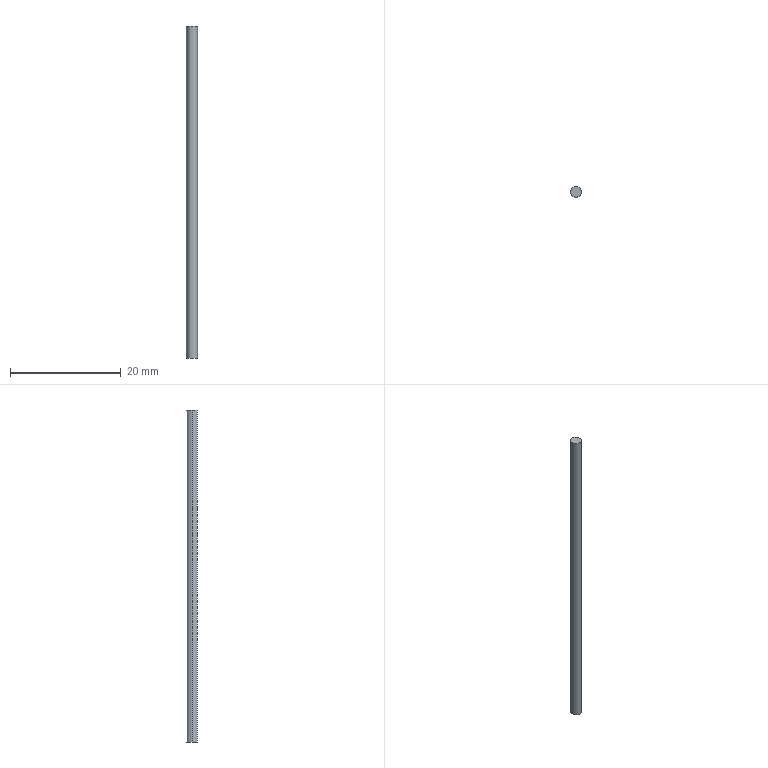Part | SolidWorks | features Extrusion 1 | 1 solid | 4 faces | box 2 x 2 x 60 mm | volume 188.496 mm3 | cylinder 2 | plane 2 | commonest cylinder face diameters 2 x2
STEP:
#1=CARTESIAN_POINT('',(1.,0.,60.));
#2=VERTEX_POINT('',#1);
#3=CARTESIAN_POINT('',(-1.,0.,60.));
#4=VERTEX_POINT('',#3);
#5=CARTESIAN_POINT('',(0.,0.,60.));
#6=DIRECTION('',(0.,0.,1.));
#7=DIRECTION('',(1.,0.,0.));
#8=AXIS2_PLACEMENT_3D('',#5,#6,#7);
#9=CIRCLE('',#8,1.);
#10=EDGE_CURVE('',#2,#4,#9,.T.);
#11=ORIENTED_EDGE('',*,*,#10,.F.);
#12=CARTESIAN_POINT('',(1.,0.,0.));
#13=VERTEX_POINT('',#12);
#14=CARTESIAN_POINT('',(1.,0.,60.));
#15=DIRECTION('',(0.,0.,-1.));
#16=VECTOR('',#15,1000.);
#17=LINE('',#14,#16);
#18=EDGE_CURVE('',#2,#13,#17,.T.);
#19=ORIENTED_EDGE('',*,*,#18,.T.);
#20=CARTESIAN_POINT('',(-1.,0.,0.));
#21=VERTEX_POINT('',#20);
#22=CARTESIAN_POINT('',(0.,0.,0.));
#23=DIRECTION('',(0.,0.,1.));
#24=DIRECTION('',(1.,0.,0.));
#25=AXIS2_PLACEMENT_3D('',#22,#23,#24);
#26=CIRCLE('',#25,1.);
#27=EDGE_CURVE('',#13,#21,#26,.T.);
#28=ORIENTED_EDGE('',*,*,#27,.T.);
#29=CARTESIAN_POINT('',(-1.,0.,60.));
#30=DIRECTION('',(0.,0.,-1.));
#31=VECTOR('',#30,1000.);
#32=LINE('',#29,#31);
#33=EDGE_CURVE('',#4,#21,#32,.T.);
#34=ORIENTED_EDGE('',*,*,#33,.F.);
#35=EDGE_LOOP('',(#11,#19,#28,#34));
#36=FACE_OUTER_BOUND('',#35,.T.);
#37=CARTESIAN_POINT('',(0.,0.,60.));
#38=DIRECTION('',(0.,0.,-1.));
#39=DIRECTION('',(-1.,0.,0.));
#40=AXIS2_PLACEMENT_3D('',#37,#38,#39);
#41=CYLINDRICAL_SURFACE('',#40,1.);
#42=ADVANCED_FACE('',(#36),#41,.T.);
#43=ORIENTED_EDGE('',*,*,#18,.F.);
#44=CARTESIAN_POINT('',(0.,0.,60.));
#45=DIRECTION('',(0.,0.,1.));
#46=DIRECTION('',(1.,0.,0.));
#47=AXIS2_PLACEMENT_3D('',#44,#45,#46);
#48=CIRCLE('',#47,1.);
#49=EDGE_CURVE('',#4,#2,#48,.T.);
#50=ORIENTED_EDGE('',*,*,#49,.F.);
#51=ORIENTED_EDGE('',*,*,#33,.T.);
#52=CARTESIAN_POINT('',(0.,0.,0.));
#53=DIRECTION('',(0.,0.,1.));
#54=DIRECTION('',(1.,0.,0.));
#55=AXIS2_PLACEMENT_3D('',#52,#53,#54);
#56=CIRCLE('',#55,1.);
#57=EDGE_CURVE('',#21,#13,#56,.T.);
#58=ORIENTED_EDGE('',*,*,#57,.T.);
#59=EDGE_LOOP('',(#43,#50,#51,#58));
#60=FACE_OUTER_BOUND('',#59,.T.);
#61=CARTESIAN_POINT('',(0.,0.,60.));
#62=DIRECTION('',(0.,0.,-1.));
#63=DIRECTION('',(-1.,0.,0.));
#64=AXIS2_PLACEMENT_3D('',#61,#62,#63);
#65=CYLINDRICAL_SURFACE('',#64,1.);
#66=ADVANCED_FACE('',(#60),#65,.T.);
#67=ORIENTED_EDGE('',*,*,#49,.T.);
#68=ORIENTED_EDGE('',*,*,#10,.T.);
#69=EDGE_LOOP('',(#67,#68));
#70=FACE_OUTER_BOUND('',#69,.T.);
#71=CARTESIAN_POINT('',(0.,0.,60.));
#72=DIRECTION('',(0.,0.,1.));
#73=DIRECTION('',(1.,0.,0.));
#74=AXIS2_PLACEMENT_3D('',#71,#72,#73);
#75=PLANE('',#74);
#76=ADVANCED_FACE('',(#70),#75,.T.);
#77=ORIENTED_EDGE('',*,*,#57,.F.);
#78=ORIENTED_EDGE('',*,*,#27,.F.);
#79=EDGE_LOOP('',(#77,#78));
#80=FACE_OUTER_BOUND('',#79,.T.);
#81=CARTESIAN_POINT('',(0.,0.,0.));
#82=DIRECTION('',(0.,0.,1.));
#83=DIRECTION('',(1.,0.,0.));
#84=AXIS2_PLACEMENT_3D('',#81,#82,#83);
#85=PLANE('',#84);
#86=ADVANCED_FACE('',(#80),#85,.F.);
#87=CLOSED_SHELL('',(#42,#66,#76,#86));
#88=MANIFOLD_SOLID_BREP('',#87);
#89=CARTESIAN_POINT('',(0.,0.,0.));
#90=DIRECTION('',(0.,0.,1.));
#91=DIRECTION('',(1.,0.,0.));
#92=AXIS2_PLACEMENT_3D('',#89,#90,#91);
#93=(LENGTH_UNIT()NAMED_UNIT(*)SI_UNIT(.MILLI.,.METRE.));
#94=UNCERTAINTY_MEASURE_WITH_UNIT(LENGTH_MEASURE(0.00001),#93,'','');
#95=(NAMED_UNIT(*)PLANE_ANGLE_UNIT()SI_UNIT($,.RADIAN.));
#96=(NAMED_UNIT(*)SI_UNIT($,.STERADIAN.)SOLID_ANGLE_UNIT());
#97=(GEOMETRIC_REPRESENTATION_CONTEXT(3)GLOBAL_UNCERTAINTY_ASSIGNED_CONTEXT((#94))GLOBAL_UNIT_ASSIGNED_CONTEXT((#93,#95,#96))REPRESENTATION_CONTEXT('',''));
#98=ADVANCED_BREP_SHAPE_REPRESENTATION('',(#88,#92),#97);